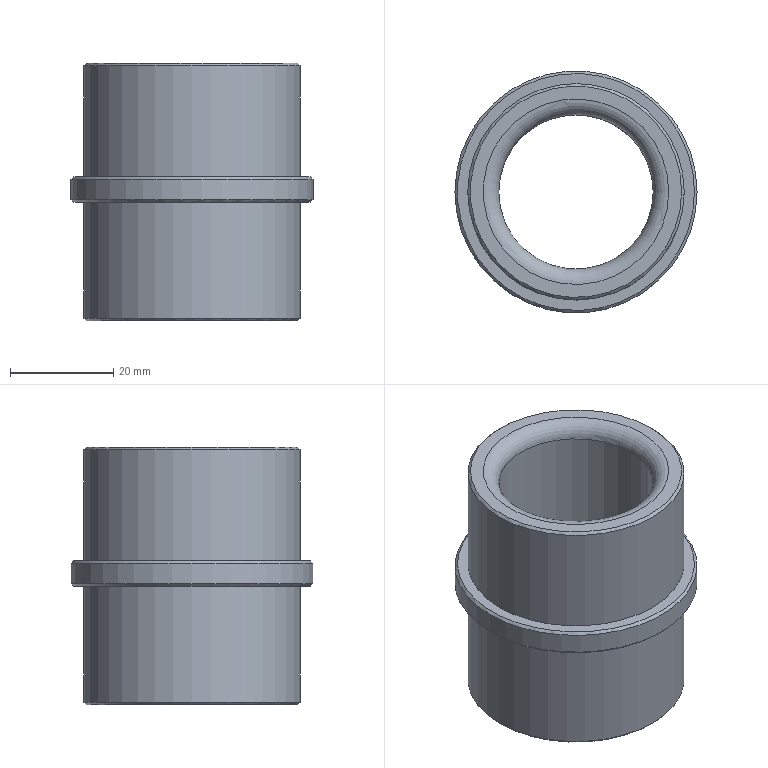Part | NX | features 模具.stp<1>[51] 2 | 1 solid | 14 faces | box 47 x 47 x 50 mm | volume 35227 mm3 | cylinder 4 | cone 4 | plane 4 | torus 2 | commonest cylinder face diameters 42 x2 30 x1 47 x1
STEP:
#1=CARTESIAN_POINT('',(178.,-265.,-193.5));
#2=VERTEX_POINT('',#1);
#3=CARTESIAN_POINT('',(160.,-265.,-193.5));
#4=DIRECTION('',(0.,0.,-1.));
#5=DIRECTION('',(1.,0.,0.));
#6=AXIS2_PLACEMENT_3D('',#3,#4,#5);
#7=CIRCLE('',#6,18.);
#8=EDGE_CURVE('',#2,#2,#7,.T.);
#9=ORIENTED_EDGE('',*,*,#8,.F.);
#10=EDGE_LOOP('',(#9));
#11=FACE_BOUND('',#10,.T.);
#12=CARTESIAN_POINT('',(175.,-265.,-196.5));
#13=VERTEX_POINT('',#12);
#14=CARTESIAN_POINT('',(160.,-265.,-196.5));
#15=DIRECTION('',(0.,0.,1.));
#16=DIRECTION('',(1.,0.,0.));
#17=AXIS2_PLACEMENT_3D('',#14,#15,#16);
#18=CIRCLE('',#17,15.);
#19=EDGE_CURVE('',#13,#13,#18,.T.);
#20=ORIENTED_EDGE('',*,*,#19,.F.);
#21=EDGE_LOOP('',(#20));
#22=FACE_BOUND('',#21,.T.);
#23=CARTESIAN_POINT('',(160.,-265.,-196.5));
#24=DIRECTION('',(0.,0.,1.));
#25=DIRECTION('',(1.,0.,0.));
#26=AXIS2_PLACEMENT_3D('',#23,#24,#25);
#27=TOROIDAL_SURFACE('',#26,18.,3.);
#28=ADVANCED_FACE('',(#11,#22),#27,.T.);
#29=CARTESIAN_POINT('',(142.,-265.,-243.5));
#30=VERTEX_POINT('',#29);
#31=CARTESIAN_POINT('',(160.,-265.,-243.5));
#32=DIRECTION('',(0.,0.,1.));
#33=DIRECTION('',(-1.,0.,0.));
#34=AXIS2_PLACEMENT_3D('',#31,#32,#33);
#35=CIRCLE('',#34,18.);
#36=EDGE_CURVE('',#30,#30,#35,.T.);
#37=ORIENTED_EDGE('',*,*,#36,.F.);
#38=EDGE_LOOP('',(#37));
#39=FACE_BOUND('',#38,.T.);
#40=CARTESIAN_POINT('',(145.,-265.,-240.5));
#41=VERTEX_POINT('',#40);
#42=CARTESIAN_POINT('',(160.,-265.,-240.5));
#43=DIRECTION('',(0.,0.,-1.));
#44=DIRECTION('',(-1.,0.,0.));
#45=AXIS2_PLACEMENT_3D('',#42,#43,#44);
#46=CIRCLE('',#45,15.);
#47=EDGE_CURVE('',#41,#41,#46,.T.);
#48=ORIENTED_EDGE('',*,*,#47,.F.);
#49=EDGE_LOOP('',(#48));
#50=FACE_BOUND('',#49,.T.);
#51=CARTESIAN_POINT('',(160.,-265.,-240.5));
#52=DIRECTION('',(0.,0.,-1.));
#53=DIRECTION('',(-1.,0.,0.));
#54=AXIS2_PLACEMENT_3D('',#51,#52,#53);
#55=TOROIDAL_SURFACE('',#54,18.,3.);
#56=ADVANCED_FACE('',(#39,#50),#55,.T.);
#57=ORIENTED_EDGE('',*,*,#19,.T.);
#58=EDGE_LOOP('',(#57));
#59=FACE_BOUND('',#58,.T.);
#60=ORIENTED_EDGE('',*,*,#47,.T.);
#61=EDGE_LOOP('',(#60));
#62=FACE_BOUND('',#61,.T.);
#63=CARTESIAN_POINT('',(160.,-265.,-243.5));
#64=DIRECTION('',(0.,0.,1.));
#65=DIRECTION('',(1.,0.,0.));
#66=AXIS2_PLACEMENT_3D('',#63,#64,#65);
#67=CYLINDRICAL_SURFACE('',#66,15.);
#68=ADVANCED_FACE('',(#59,#62),#67,.F.);
#69=CARTESIAN_POINT('',(139.,-265.,-243.));
#70=VERTEX_POINT('',#69);
#71=CARTESIAN_POINT('',(160.,-265.,-243.));
#72=DIRECTION('',(0.,0.,1.));
#73=DIRECTION('',(-1.,0.,0.));
#74=AXIS2_PLACEMENT_3D('',#71,#72,#73);
#75=CIRCLE('',#74,21.);
#76=EDGE_CURVE('',#70,#70,#75,.T.);
#77=ORIENTED_EDGE('',*,*,#76,.T.);
#78=EDGE_LOOP('',(#77));
#79=FACE_BOUND('',#78,.T.);
#80=CARTESIAN_POINT('',(139.,-265.,-220.5));
#81=VERTEX_POINT('',#80);
#82=CARTESIAN_POINT('',(160.,-265.,-220.5));
#83=DIRECTION('',(0.,0.,1.));
#84=DIRECTION('',(-1.,0.,0.));
#85=AXIS2_PLACEMENT_3D('',#82,#83,#84);
#86=CIRCLE('',#85,21.);
#87=EDGE_CURVE('',#81,#81,#86,.T.);
#88=ORIENTED_EDGE('',*,*,#87,.F.);
#89=EDGE_LOOP('',(#88));
#90=FACE_BOUND('',#89,.T.);
#91=CARTESIAN_POINT('',(160.,-265.,-243.5));
#92=DIRECTION('',(0.,0.,1.));
#93=DIRECTION('',(1.,0.,0.));
#94=AXIS2_PLACEMENT_3D('',#91,#92,#93);
#95=CYLINDRICAL_SURFACE('',#94,21.);
#96=ADVANCED_FACE('',(#79,#90),#95,.T.);
#97=ORIENTED_EDGE('',*,*,#76,.F.);
#98=EDGE_LOOP('',(#97));
#99=FACE_BOUND('',#98,.T.);
#100=CARTESIAN_POINT('',(139.5,-265.,-243.5));
#101=VERTEX_POINT('',#100);
#102=CARTESIAN_POINT('',(160.,-265.,-243.5));
#103=DIRECTION('',(0.,0.,-1.));
#104=DIRECTION('',(-1.,0.,0.));
#105=AXIS2_PLACEMENT_3D('',#102,#103,#104);
#106=CIRCLE('',#105,20.5);
#107=EDGE_CURVE('',#101,#101,#106,.T.);
#108=ORIENTED_EDGE('',*,*,#107,.F.);
#109=EDGE_LOOP('',(#108));
#110=FACE_BOUND('',#109,.T.);
#111=CARTESIAN_POINT('',(160.,-265.,-243.));
#112=DIRECTION('',(0.,0.,1.));
#113=DIRECTION('',(1.,0.,0.));
#114=AXIS2_PLACEMENT_3D('',#111,#112,#113);
#115=CONICAL_SURFACE('',#114,21.,0.7854);
#116=ADVANCED_FACE('',(#99,#110),#115,.T.);
#117=ORIENTED_EDGE('',*,*,#107,.T.);
#118=EDGE_LOOP('',(#117));
#119=FACE_BOUND('',#118,.T.);
#120=ORIENTED_EDGE('',*,*,#36,.T.);
#121=EDGE_LOOP('',(#120));
#122=FACE_BOUND('',#121,.T.);
#123=CARTESIAN_POINT('',(160.,-265.,-243.5));
#124=DIRECTION('',(0.,0.,-1.));
#125=DIRECTION('',(0.,-1.,0.));
#126=AXIS2_PLACEMENT_3D('',#123,#124,#125);
#127=PLANE('',#126);
#128=ADVANCED_FACE('',(#119,#122),#127,.T.);
#129=CARTESIAN_POINT('',(183.5,-265.,-216.));
#130=VERTEX_POINT('',#129);
#131=CARTESIAN_POINT('',(160.,-265.,-216.));
#132=DIRECTION('',(0.,0.,-1.));
#133=DIRECTION('',(1.,0.,0.));
#134=AXIS2_PLACEMENT_3D('',#131,#132,#133);
#135=CIRCLE('',#134,23.5);
#136=EDGE_CURVE('',#130,#130,#135,.T.);
#137=ORIENTED_EDGE('',*,*,#136,.F.);
#138=EDGE_LOOP('',(#137));
#139=FACE_BOUND('',#138,.T.);
#140=CARTESIAN_POINT('',(183.,-265.,-215.5));
#141=VERTEX_POINT('',#140);
#142=CARTESIAN_POINT('',(160.,-265.,-215.5));
#143=DIRECTION('',(0.,0.,1.));
#144=DIRECTION('',(1.,0.,0.));
#145=AXIS2_PLACEMENT_3D('',#142,#143,#144);
#146=CIRCLE('',#145,23.);
#147=EDGE_CURVE('',#141,#141,#146,.T.);
#148=ORIENTED_EDGE('',*,*,#147,.F.);
#149=EDGE_LOOP('',(#148));
#150=FACE_BOUND('',#149,.T.);
#151=CARTESIAN_POINT('',(160.,-265.,-216.));
#152=DIRECTION('',(0.,0.,-1.));
#153=DIRECTION('',(-1.,0.,0.));
#154=AXIS2_PLACEMENT_3D('',#151,#152,#153);
#155=CONICAL_SURFACE('',#154,23.5,0.7854);
#156=ADVANCED_FACE('',(#139,#150),#155,.T.);
#157=CARTESIAN_POINT('',(136.5,-265.,-220.));
#158=VERTEX_POINT('',#157);
#159=CARTESIAN_POINT('',(160.,-265.,-220.));
#160=DIRECTION('',(0.,0.,1.));
#161=DIRECTION('',(-1.,0.,0.));
#162=AXIS2_PLACEMENT_3D('',#159,#160,#161);
#163=CIRCLE('',#162,23.5);
#164=EDGE_CURVE('',#158,#158,#163,.T.);
#165=ORIENTED_EDGE('',*,*,#164,.F.);
#166=EDGE_LOOP('',(#165));
#167=FACE_BOUND('',#166,.T.);
#168=CARTESIAN_POINT('',(137.,-265.,-220.5));
#169=VERTEX_POINT('',#168);
#170=CARTESIAN_POINT('',(160.,-265.,-220.5));
#171=DIRECTION('',(0.,0.,-1.));
#172=DIRECTION('',(-1.,0.,0.));
#173=AXIS2_PLACEMENT_3D('',#170,#171,#172);
#174=CIRCLE('',#173,23.);
#175=EDGE_CURVE('',#169,#169,#174,.T.);
#176=ORIENTED_EDGE('',*,*,#175,.F.);
#177=EDGE_LOOP('',(#176));
#178=FACE_BOUND('',#177,.T.);
#179=CARTESIAN_POINT('',(160.,-265.,-220.));
#180=DIRECTION('',(0.,0.,1.));
#181=DIRECTION('',(1.,0.,0.));
#182=AXIS2_PLACEMENT_3D('',#179,#180,#181);
#183=CONICAL_SURFACE('',#182,23.5,0.7854);
#184=ADVANCED_FACE('',(#167,#178),#183,.T.);
#185=ORIENTED_EDGE('',*,*,#136,.T.);
#186=EDGE_LOOP('',(#185));
#187=FACE_BOUND('',#186,.T.);
#188=ORIENTED_EDGE('',*,*,#164,.T.);
#189=EDGE_LOOP('',(#188));
#190=FACE_BOUND('',#189,.T.);
#191=CARTESIAN_POINT('',(160.,-265.,-220.5));
#192=DIRECTION('',(0.,0.,1.));
#193=DIRECTION('',(1.,0.,0.));
#194=AXIS2_PLACEMENT_3D('',#191,#192,#193);
#195=CYLINDRICAL_SURFACE('',#194,23.5);
#196=ADVANCED_FACE('',(#187,#190),#195,.T.);
#197=ORIENTED_EDGE('',*,*,#175,.T.);
#198=EDGE_LOOP('',(#197));
#199=FACE_BOUND('',#198,.T.);
#200=ORIENTED_EDGE('',*,*,#87,.T.);
#201=EDGE_LOOP('',(#200));
#202=FACE_BOUND('',#201,.T.);
#203=CARTESIAN_POINT('',(160.,-265.,-220.5));
#204=DIRECTION('',(0.,0.,-1.));
#205=DIRECTION('',(0.,-1.,0.));
#206=AXIS2_PLACEMENT_3D('',#203,#204,#205);
#207=PLANE('',#206);
#208=ADVANCED_FACE('',(#199,#202),#207,.T.);
#209=ORIENTED_EDGE('',*,*,#147,.T.);
#210=EDGE_LOOP('',(#209));
#211=FACE_BOUND('',#210,.T.);
#212=CARTESIAN_POINT('',(181.,-265.,-215.5));
#213=VERTEX_POINT('',#212);
#214=CARTESIAN_POINT('',(160.,-265.,-215.5));
#215=DIRECTION('',(0.,0.,-1.));
#216=DIRECTION('',(1.,0.,0.));
#217=AXIS2_PLACEMENT_3D('',#214,#215,#216);
#218=CIRCLE('',#217,21.);
#219=EDGE_CURVE('',#213,#213,#218,.T.);
#220=ORIENTED_EDGE('',*,*,#219,.T.);
#221=EDGE_LOOP('',(#220));
#222=FACE_BOUND('',#221,.T.);
#223=CARTESIAN_POINT('',(160.,-265.,-215.5));
#224=DIRECTION('',(0.,0.,1.));
#225=DIRECTION('',(1.,0.,0.));
#226=AXIS2_PLACEMENT_3D('',#223,#224,#225);
#227=PLANE('',#226);
#228=ADVANCED_FACE('',(#211,#222),#227,.T.);
#229=CARTESIAN_POINT('',(181.,-265.,-194.));
#230=VERTEX_POINT('',#229);
#231=CARTESIAN_POINT('',(160.,-265.,-194.));
#232=DIRECTION('',(0.,0.,-1.));
#233=DIRECTION('',(1.,0.,0.));
#234=AXIS2_PLACEMENT_3D('',#231,#232,#233);
#235=CIRCLE('',#234,21.);
#236=EDGE_CURVE('',#230,#230,#235,.T.);
#237=ORIENTED_EDGE('',*,*,#236,.F.);
#238=EDGE_LOOP('',(#237));
#239=FACE_BOUND('',#238,.T.);
#240=CARTESIAN_POINT('',(180.5,-265.,-193.5));
#241=VERTEX_POINT('',#240);
#242=CARTESIAN_POINT('',(160.,-265.,-193.5));
#243=DIRECTION('',(0.,0.,1.));
#244=DIRECTION('',(1.,0.,0.));
#245=AXIS2_PLACEMENT_3D('',#242,#243,#244);
#246=CIRCLE('',#245,20.5);
#247=EDGE_CURVE('',#241,#241,#246,.T.);
#248=ORIENTED_EDGE('',*,*,#247,.F.);
#249=EDGE_LOOP('',(#248));
#250=FACE_BOUND('',#249,.T.);
#251=CARTESIAN_POINT('',(160.,-265.,-194.));
#252=DIRECTION('',(0.,0.,-1.));
#253=DIRECTION('',(-1.,0.,0.));
#254=AXIS2_PLACEMENT_3D('',#251,#252,#253);
#255=CONICAL_SURFACE('',#254,21.,0.7854);
#256=ADVANCED_FACE('',(#239,#250),#255,.T.);
#257=ORIENTED_EDGE('',*,*,#247,.T.);
#258=EDGE_LOOP('',(#257));
#259=FACE_BOUND('',#258,.T.);
#260=ORIENTED_EDGE('',*,*,#8,.T.);
#261=EDGE_LOOP('',(#260));
#262=FACE_BOUND('',#261,.T.);
#263=CARTESIAN_POINT('',(160.,-265.,-193.5));
#264=DIRECTION('',(0.,0.,1.));
#265=DIRECTION('',(1.,0.,0.));
#266=AXIS2_PLACEMENT_3D('',#263,#264,#265);
#267=PLANE('',#266);
#268=ADVANCED_FACE('',(#259,#262),#267,.T.);
#269=ORIENTED_EDGE('',*,*,#236,.T.);
#270=EDGE_LOOP('',(#269));
#271=FACE_BOUND('',#270,.T.);
#272=ORIENTED_EDGE('',*,*,#219,.F.);
#273=EDGE_LOOP('',(#272));
#274=FACE_BOUND('',#273,.T.);
#275=CARTESIAN_POINT('',(160.,-265.,-243.5));
#276=DIRECTION('',(0.,0.,1.));
#277=DIRECTION('',(1.,0.,0.));
#278=AXIS2_PLACEMENT_3D('',#275,#276,#277);
#279=CYLINDRICAL_SURFACE('',#278,21.);
#280=ADVANCED_FACE('',(#271,#274),#279,.T.);
#281=CLOSED_SHELL('',(#28,#56,#68,#96,#116,#128,#156,#184,#196,#208,#228,#256,#268,#280));
#282=MANIFOLD_SOLID_BREP('',#281);
#283=(LENGTH_UNIT()NAMED_UNIT(*)SI_UNIT(.MILLI.,.METRE.));
#284=UNCERTAINTY_MEASURE_WITH_UNIT(LENGTH_MEASURE(0.00001),#283,'','');
#285=(NAMED_UNIT(*)PLANE_ANGLE_UNIT()SI_UNIT($,.RADIAN.));
#286=(NAMED_UNIT(*)SI_UNIT($,.STERADIAN.)SOLID_ANGLE_UNIT());
#287=(GEOMETRIC_REPRESENTATION_CONTEXT(3)GLOBAL_UNCERTAINTY_ASSIGNED_CONTEXT((#284))GLOBAL_UNIT_ASSIGNED_CONTEXT((#283,#285,#286))REPRESENTATION_CONTEXT('',''));
#288=ADVANCED_BREP_SHAPE_REPRESENTATION('',(#282),#287);